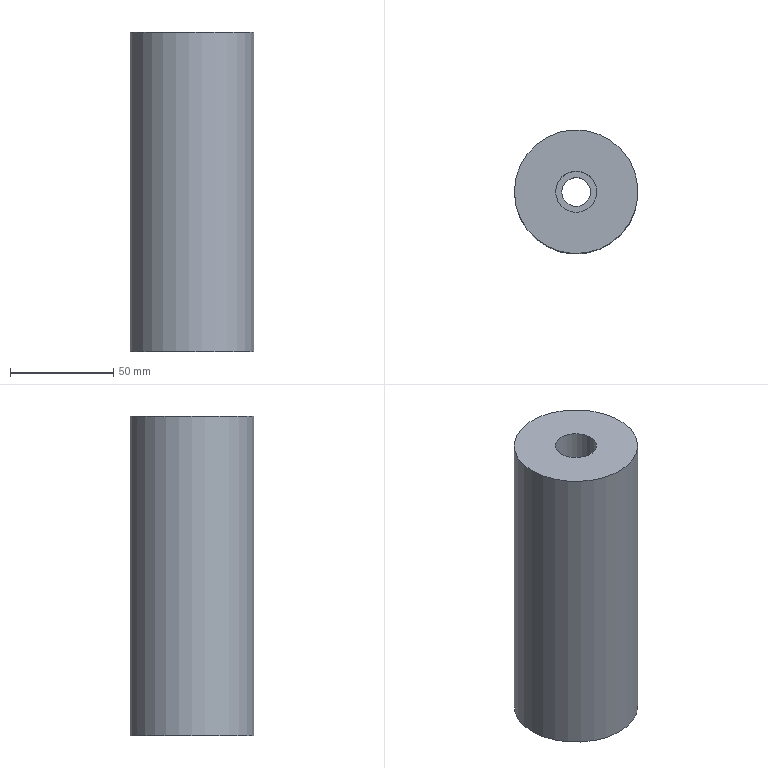Part | NX | features solid 2 | 1 solid | 6 faces | box 60 x 60 x 155 mm | volume 402375 mm3 | plane 3 | cylinder 3 | commonest cylinder face diameters 14 x1 20 x1 60 x1
STEP:
#1=CARTESIAN_POINT('',(1090.,-845.,125.));
#2=VERTEX_POINT('',#1);
#3=CARTESIAN_POINT('',(1120.,-845.,125.));
#4=DIRECTION('',(0.,0.,-1.));
#5=DIRECTION('',(-1.,0.,0.));
#6=AXIS2_PLACEMENT_3D('',#3,#4,#5);
#7=CIRCLE('',#6,30.);
#8=EDGE_CURVE('',#2,#2,#7,.T.);
#9=ORIENTED_EDGE('',*,*,#8,.F.);
#10=EDGE_LOOP('',(#9));
#11=FACE_BOUND('',#10,.T.);
#12=CARTESIAN_POINT('',(1110.,-845.,125.));
#13=VERTEX_POINT('',#12);
#14=CARTESIAN_POINT('',(1120.,-845.,125.));
#15=DIRECTION('',(0.,0.,-1.));
#16=DIRECTION('',(-1.,0.,0.));
#17=AXIS2_PLACEMENT_3D('',#14,#15,#16);
#18=CIRCLE('',#17,10.);
#19=EDGE_CURVE('',#13,#13,#18,.T.);
#20=ORIENTED_EDGE('',*,*,#19,.T.);
#21=EDGE_LOOP('',(#20));
#22=FACE_BOUND('',#21,.T.);
#23=CARTESIAN_POINT('',(1120.,-845.,125.));
#24=DIRECTION('',(0.,0.,1.));
#25=DIRECTION('',(-1.,0.,0.));
#26=AXIS2_PLACEMENT_3D('',#23,#24,#25);
#27=PLANE('',#26);
#28=ADVANCED_FACE('',(#11,#22),#27,.T.);
#29=CARTESIAN_POINT('',(1113.,-845.,-30.));
#30=VERTEX_POINT('',#29);
#31=CARTESIAN_POINT('',(1120.,-845.,-30.));
#32=DIRECTION('',(0.,0.,-1.));
#33=DIRECTION('',(-1.,0.,0.));
#34=AXIS2_PLACEMENT_3D('',#31,#32,#33);
#35=CIRCLE('',#34,7.);
#36=EDGE_CURVE('',#30,#30,#35,.T.);
#37=ORIENTED_EDGE('',*,*,#36,.T.);
#38=EDGE_LOOP('',(#37));
#39=FACE_BOUND('',#38,.T.);
#40=CARTESIAN_POINT('',(1113.,-845.,50.));
#41=VERTEX_POINT('',#40);
#42=CARTESIAN_POINT('',(1120.,-845.,50.));
#43=DIRECTION('',(0.,0.,-1.));
#44=DIRECTION('',(-1.,0.,0.));
#45=AXIS2_PLACEMENT_3D('',#42,#43,#44);
#46=CIRCLE('',#45,7.);
#47=EDGE_CURVE('',#41,#41,#46,.T.);
#48=ORIENTED_EDGE('',*,*,#47,.F.);
#49=EDGE_LOOP('',(#48));
#50=FACE_BOUND('',#49,.T.);
#51=CARTESIAN_POINT('',(1120.,-845.,125.));
#52=DIRECTION('',(0.,0.,-1.));
#53=DIRECTION('',(1.,0.,0.));
#54=AXIS2_PLACEMENT_3D('',#51,#52,#53);
#55=CYLINDRICAL_SURFACE('',#54,7.);
#56=ADVANCED_FACE('',(#39,#50),#55,.F.);
#57=CARTESIAN_POINT('',(1090.,-845.,-30.));
#58=VERTEX_POINT('',#57);
#59=CARTESIAN_POINT('',(1120.,-845.,-30.));
#60=DIRECTION('',(0.,0.,-1.));
#61=DIRECTION('',(-1.,0.,0.));
#62=AXIS2_PLACEMENT_3D('',#59,#60,#61);
#63=CIRCLE('',#62,30.);
#64=EDGE_CURVE('',#58,#58,#63,.T.);
#65=ORIENTED_EDGE('',*,*,#64,.T.);
#66=EDGE_LOOP('',(#65));
#67=FACE_BOUND('',#66,.T.);
#68=ORIENTED_EDGE('',*,*,#36,.F.);
#69=EDGE_LOOP('',(#68));
#70=FACE_BOUND('',#69,.T.);
#71=CARTESIAN_POINT('',(1120.,-845.,-30.));
#72=DIRECTION('',(0.,0.,1.));
#73=DIRECTION('',(-1.,0.,0.));
#74=AXIS2_PLACEMENT_3D('',#71,#72,#73);
#75=PLANE('',#74);
#76=ADVANCED_FACE('',(#67,#70),#75,.F.);
#77=ORIENTED_EDGE('',*,*,#8,.T.);
#78=EDGE_LOOP('',(#77));
#79=FACE_BOUND('',#78,.T.);
#80=ORIENTED_EDGE('',*,*,#64,.F.);
#81=EDGE_LOOP('',(#80));
#82=FACE_BOUND('',#81,.T.);
#83=CARTESIAN_POINT('',(1120.,-845.,125.));
#84=DIRECTION('',(0.,0.,-1.));
#85=DIRECTION('',(1.,0.,0.));
#86=AXIS2_PLACEMENT_3D('',#83,#84,#85);
#87=CYLINDRICAL_SURFACE('',#86,30.);
#88=ADVANCED_FACE('',(#79,#82),#87,.T.);
#89=ORIENTED_EDGE('',*,*,#19,.F.);
#90=EDGE_LOOP('',(#89));
#91=FACE_BOUND('',#90,.T.);
#92=CARTESIAN_POINT('',(1110.,-845.,50.));
#93=VERTEX_POINT('',#92);
#94=CARTESIAN_POINT('',(1120.,-845.,50.));
#95=DIRECTION('',(0.,0.,-1.));
#96=DIRECTION('',(-1.,0.,0.));
#97=AXIS2_PLACEMENT_3D('',#94,#95,#96);
#98=CIRCLE('',#97,10.);
#99=EDGE_CURVE('',#93,#93,#98,.T.);
#100=ORIENTED_EDGE('',*,*,#99,.T.);
#101=EDGE_LOOP('',(#100));
#102=FACE_BOUND('',#101,.T.);
#103=CARTESIAN_POINT('',(1120.,-845.,125.));
#104=DIRECTION('',(0.,0.,-1.));
#105=DIRECTION('',(1.,0.,0.));
#106=AXIS2_PLACEMENT_3D('',#103,#104,#105);
#107=CYLINDRICAL_SURFACE('',#106,10.);
#108=ADVANCED_FACE('',(#91,#102),#107,.F.);
#109=ORIENTED_EDGE('',*,*,#47,.T.);
#110=EDGE_LOOP('',(#109));
#111=FACE_BOUND('',#110,.T.);
#112=ORIENTED_EDGE('',*,*,#99,.F.);
#113=EDGE_LOOP('',(#112));
#114=FACE_BOUND('',#113,.T.);
#115=CARTESIAN_POINT('',(1120.,-845.,50.));
#116=DIRECTION('',(0.,0.,1.));
#117=DIRECTION('',(-1.,0.,0.));
#118=AXIS2_PLACEMENT_3D('',#115,#116,#117);
#119=PLANE('',#118);
#120=ADVANCED_FACE('',(#111,#114),#119,.T.);
#121=CLOSED_SHELL('',(#28,#56,#76,#88,#108,#120));
#122=MANIFOLD_SOLID_BREP('',#121);
#123=(LENGTH_UNIT()NAMED_UNIT(*)SI_UNIT(.MILLI.,.METRE.));
#124=UNCERTAINTY_MEASURE_WITH_UNIT(LENGTH_MEASURE(0.00001),#123,'','');
#125=(NAMED_UNIT(*)PLANE_ANGLE_UNIT()SI_UNIT($,.RADIAN.));
#126=(NAMED_UNIT(*)SI_UNIT($,.STERADIAN.)SOLID_ANGLE_UNIT());
#127=(GEOMETRIC_REPRESENTATION_CONTEXT(3)GLOBAL_UNCERTAINTY_ASSIGNED_CONTEXT((#124))GLOBAL_UNIT_ASSIGNED_CONTEXT((#123,#125,#126))REPRESENTATION_CONTEXT('',''));
#128=ADVANCED_BREP_SHAPE_REPRESENTATION('',(#122),#127);